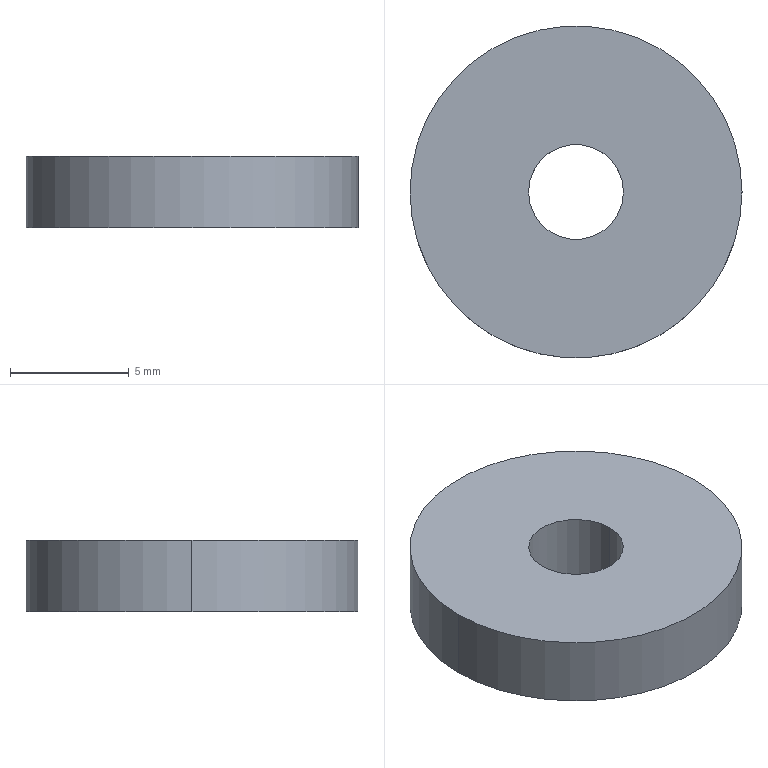Part | NX | 1 solid | 6 faces | box 14 x 14 x 3 mm | volume 424.115 mm3 | cylinder 4 | plane 2 | commonest cylinder face diameters 4 x2 14 x2
STEP:
#1=CARTESIAN_POINT('',(-7.,0.,0.));
#2=VERTEX_POINT('',#1);
#3=CARTESIAN_POINT('',(7.,0.,0.));
#4=VERTEX_POINT('',#3);
#5=CARTESIAN_POINT('',(0.,0.,0.));
#6=DIRECTION('',(0.,0.,1.));
#7=DIRECTION('',(-1.,0.,0.));
#8=AXIS2_PLACEMENT_3D('',#5,#6,#7);
#9=CIRCLE('',#8,7.);
#10=EDGE_CURVE('',#2,#4,#9,.T.);
#11=ORIENTED_EDGE('',*,*,#10,.F.);
#12=CARTESIAN_POINT('',(0.,0.,0.));
#13=DIRECTION('',(0.,0.,1.));
#14=DIRECTION('',(-1.,0.,0.));
#15=AXIS2_PLACEMENT_3D('',#12,#13,#14);
#16=CIRCLE('',#15,7.);
#17=EDGE_CURVE('',#4,#2,#16,.T.);
#18=ORIENTED_EDGE('',*,*,#17,.F.);
#19=EDGE_LOOP('',(#11,#18));
#20=FACE_BOUND('',#19,.T.);
#21=CARTESIAN_POINT('',(2.,0.,0.));
#22=VERTEX_POINT('',#21);
#23=CARTESIAN_POINT('',(-2.,0.,0.));
#24=VERTEX_POINT('',#23);
#25=CARTESIAN_POINT('',(0.,0.,0.));
#26=DIRECTION('',(0.,0.,-1.));
#27=DIRECTION('',(-1.,0.,0.));
#28=AXIS2_PLACEMENT_3D('',#25,#26,#27);
#29=CIRCLE('',#28,2.);
#30=EDGE_CURVE('',#22,#24,#29,.T.);
#31=ORIENTED_EDGE('',*,*,#30,.F.);
#32=CARTESIAN_POINT('',(0.,0.,0.));
#33=DIRECTION('',(0.,0.,-1.));
#34=DIRECTION('',(-1.,0.,0.));
#35=AXIS2_PLACEMENT_3D('',#32,#33,#34);
#36=CIRCLE('',#35,2.);
#37=EDGE_CURVE('',#24,#22,#36,.T.);
#38=ORIENTED_EDGE('',*,*,#37,.F.);
#39=EDGE_LOOP('',(#31,#38));
#40=FACE_BOUND('',#39,.T.);
#41=CARTESIAN_POINT('',(0.,0.,0.));
#42=DIRECTION('',(0.,0.,1.));
#43=DIRECTION('',(1.,0.,0.));
#44=AXIS2_PLACEMENT_3D('',#41,#42,#43);
#45=PLANE('',#44);
#46=ADVANCED_FACE('',(#20,#40),#45,.F.);
#47=CARTESIAN_POINT('',(7.,0.,3.));
#48=VERTEX_POINT('',#47);
#49=CARTESIAN_POINT('',(-7.,0.,3.));
#50=VERTEX_POINT('',#49);
#51=CARTESIAN_POINT('',(0.,0.,3.));
#52=DIRECTION('',(0.,0.,-1.));
#53=DIRECTION('',(-1.,0.,0.));
#54=AXIS2_PLACEMENT_3D('',#51,#52,#53);
#55=CIRCLE('',#54,7.);
#56=EDGE_CURVE('',#48,#50,#55,.T.);
#57=ORIENTED_EDGE('',*,*,#56,.T.);
#58=CARTESIAN_POINT('',(-7.,0.,0.));
#59=DIRECTION('',(0.,0.,1.));
#60=VECTOR('',#59,1000.);
#61=LINE('',#58,#60);
#62=EDGE_CURVE('',#2,#50,#61,.T.);
#63=ORIENTED_EDGE('',*,*,#62,.F.);
#64=ORIENTED_EDGE('',*,*,#10,.T.);
#65=CARTESIAN_POINT('',(7.,0.,0.));
#66=DIRECTION('',(0.,0.,1.));
#67=VECTOR('',#66,1000.);
#68=LINE('',#65,#67);
#69=EDGE_CURVE('',#4,#48,#68,.T.);
#70=ORIENTED_EDGE('',*,*,#69,.T.);
#71=EDGE_LOOP('',(#57,#63,#64,#70));
#72=FACE_BOUND('',#71,.T.);
#73=CARTESIAN_POINT('',(0.,0.,0.));
#74=DIRECTION('',(0.,0.,1.));
#75=DIRECTION('',(1.,0.,0.));
#76=AXIS2_PLACEMENT_3D('',#73,#74,#75);
#77=CYLINDRICAL_SURFACE('',#76,7.);
#78=ADVANCED_FACE('',(#72),#77,.T.);
#79=CARTESIAN_POINT('',(2.,0.,3.));
#80=VERTEX_POINT('',#79);
#81=CARTESIAN_POINT('',(-2.,0.,3.));
#82=VERTEX_POINT('',#81);
#83=CARTESIAN_POINT('',(0.,0.,3.));
#84=DIRECTION('',(0.,0.,1.));
#85=DIRECTION('',(1.,0.,0.));
#86=AXIS2_PLACEMENT_3D('',#83,#84,#85);
#87=CIRCLE('',#86,2.);
#88=EDGE_CURVE('',#80,#82,#87,.T.);
#89=ORIENTED_EDGE('',*,*,#88,.T.);
#90=CARTESIAN_POINT('',(-2.,0.,0.));
#91=DIRECTION('',(0.,0.,1.));
#92=VECTOR('',#91,1000.);
#93=LINE('',#90,#92);
#94=EDGE_CURVE('',#82,#24,#93,.F.);
#95=ORIENTED_EDGE('',*,*,#94,.T.);
#96=ORIENTED_EDGE('',*,*,#37,.T.);
#97=CARTESIAN_POINT('',(2.,0.,0.));
#98=DIRECTION('',(0.,0.,1.));
#99=VECTOR('',#98,1000.);
#100=LINE('',#97,#99);
#101=EDGE_CURVE('',#80,#22,#100,.F.);
#102=ORIENTED_EDGE('',*,*,#101,.F.);
#103=EDGE_LOOP('',(#89,#95,#96,#102));
#104=FACE_BOUND('',#103,.T.);
#105=CARTESIAN_POINT('',(0.,0.,0.));
#106=DIRECTION('',(0.,0.,1.));
#107=DIRECTION('',(1.,0.,0.));
#108=AXIS2_PLACEMENT_3D('',#105,#106,#107);
#109=CYLINDRICAL_SURFACE('',#108,2.);
#110=ADVANCED_FACE('',(#104),#109,.F.);
#111=ORIENTED_EDGE('',*,*,#56,.F.);
#112=CARTESIAN_POINT('',(0.,0.,3.));
#113=DIRECTION('',(0.,0.,-1.));
#114=DIRECTION('',(-1.,0.,0.));
#115=AXIS2_PLACEMENT_3D('',#112,#113,#114);
#116=CIRCLE('',#115,7.);
#117=EDGE_CURVE('',#50,#48,#116,.T.);
#118=ORIENTED_EDGE('',*,*,#117,.F.);
#119=EDGE_LOOP('',(#111,#118));
#120=FACE_BOUND('',#119,.T.);
#121=ORIENTED_EDGE('',*,*,#88,.F.);
#122=CARTESIAN_POINT('',(0.,0.,3.));
#123=DIRECTION('',(0.,0.,1.));
#124=DIRECTION('',(1.,0.,0.));
#125=AXIS2_PLACEMENT_3D('',#122,#123,#124);
#126=CIRCLE('',#125,2.);
#127=EDGE_CURVE('',#82,#80,#126,.T.);
#128=ORIENTED_EDGE('',*,*,#127,.F.);
#129=EDGE_LOOP('',(#121,#128));
#130=FACE_BOUND('',#129,.T.);
#131=CARTESIAN_POINT('',(0.,0.,3.));
#132=DIRECTION('',(0.,0.,1.));
#133=DIRECTION('',(1.,0.,0.));
#134=AXIS2_PLACEMENT_3D('',#131,#132,#133);
#135=PLANE('',#134);
#136=ADVANCED_FACE('',(#120,#130),#135,.T.);
#137=ORIENTED_EDGE('',*,*,#69,.F.);
#138=ORIENTED_EDGE('',*,*,#17,.T.);
#139=ORIENTED_EDGE('',*,*,#62,.T.);
#140=ORIENTED_EDGE('',*,*,#117,.T.);
#141=EDGE_LOOP('',(#137,#138,#139,#140));
#142=FACE_BOUND('',#141,.T.);
#143=CARTESIAN_POINT('',(0.,0.,0.));
#144=DIRECTION('',(0.,0.,1.));
#145=DIRECTION('',(1.,0.,0.));
#146=AXIS2_PLACEMENT_3D('',#143,#144,#145);
#147=CYLINDRICAL_SURFACE('',#146,7.);
#148=ADVANCED_FACE('',(#142),#147,.T.);
#149=ORIENTED_EDGE('',*,*,#30,.T.);
#150=ORIENTED_EDGE('',*,*,#94,.F.);
#151=ORIENTED_EDGE('',*,*,#127,.T.);
#152=ORIENTED_EDGE('',*,*,#101,.T.);
#153=EDGE_LOOP('',(#149,#150,#151,#152));
#154=FACE_BOUND('',#153,.T.);
#155=CARTESIAN_POINT('',(0.,0.,0.));
#156=DIRECTION('',(0.,0.,1.));
#157=DIRECTION('',(1.,0.,0.));
#158=AXIS2_PLACEMENT_3D('',#155,#156,#157);
#159=CYLINDRICAL_SURFACE('',#158,2.);
#160=ADVANCED_FACE('',(#154),#159,.F.);
#161=CLOSED_SHELL('',(#46,#78,#110,#136,#148,#160));
#162=MANIFOLD_SOLID_BREP('',#161);
#163=(LENGTH_UNIT()NAMED_UNIT(*)SI_UNIT(.MILLI.,.METRE.));
#164=UNCERTAINTY_MEASURE_WITH_UNIT(LENGTH_MEASURE(0.00001),#163,'','');
#165=(NAMED_UNIT(*)PLANE_ANGLE_UNIT()SI_UNIT($,.RADIAN.));
#166=(NAMED_UNIT(*)SI_UNIT($,.STERADIAN.)SOLID_ANGLE_UNIT());
#167=(GEOMETRIC_REPRESENTATION_CONTEXT(3)GLOBAL_UNCERTAINTY_ASSIGNED_CONTEXT((#164))GLOBAL_UNIT_ASSIGNED_CONTEXT((#163,#165,#166))REPRESENTATION_CONTEXT('',''));
#168=ADVANCED_BREP_SHAPE_REPRESENTATION('',(#162),#167);